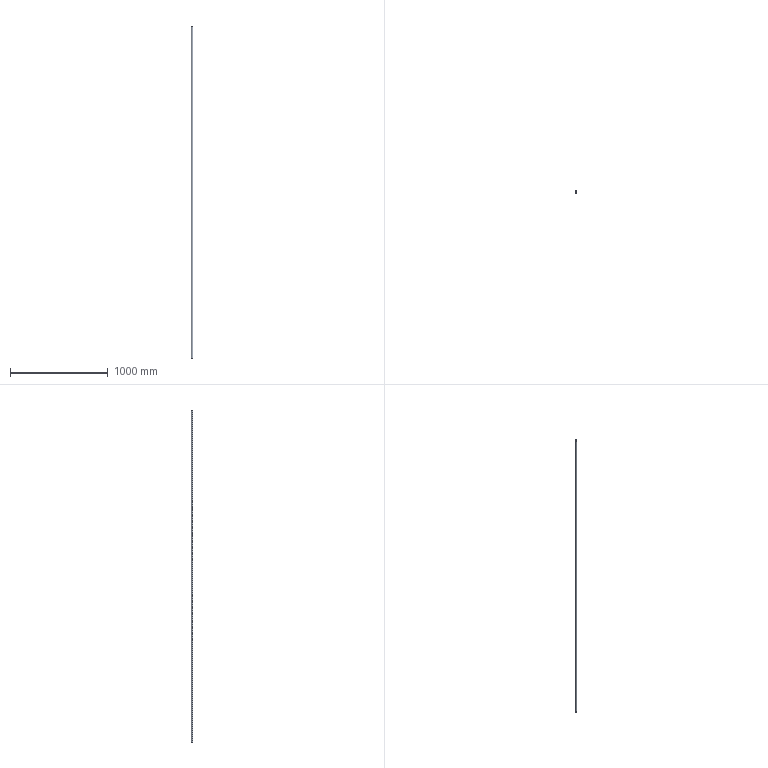Part | STEP file | BCC3 H16_13 | 1 solid | 21 faces | box 20 x 20 x 3390 mm | volume 1063554 mm3 | plane 11 | cylinder 10 | commonest cylinder face diameters 5 x8 20 x2